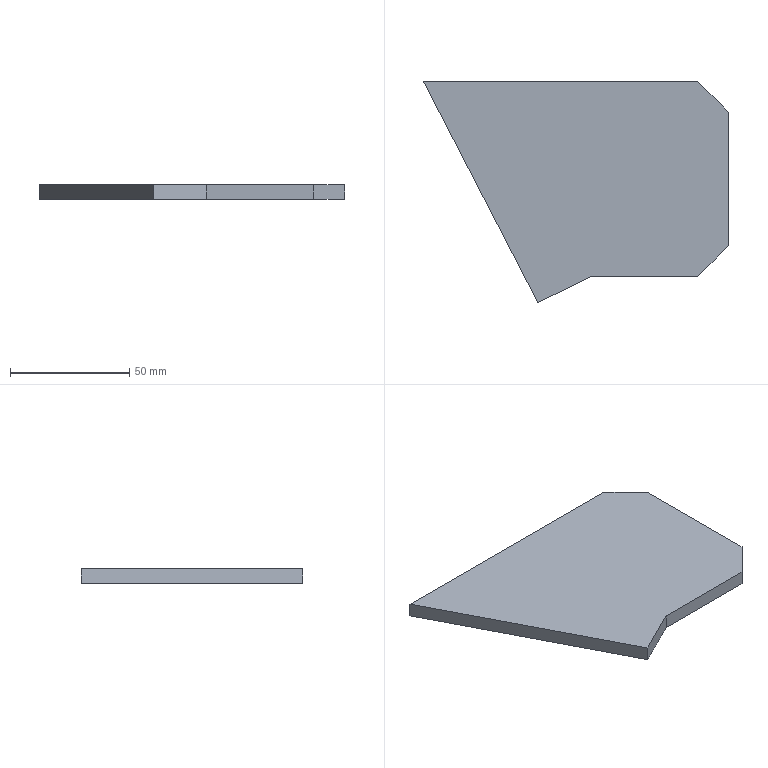Part | SolidWorks | features FlatPattern 1, SMBaseFlange 1, SheetMetal 1 | 1 solid | 9 faces | box 128 x 93 x 6 mm | volume 52464 mm3 | plane 9
STEP:
#1=CARTESIAN_POINT('',(0.,0.,0.));
#2=VERTEX_POINT('',#1);
#3=CARTESIAN_POINT('',(48.,-93.,0.));
#4=VERTEX_POINT('',#3);
#5=CARTESIAN_POINT('',(48.,-93.,0.));
#6=DIRECTION('',(0.4586,-0.8886,0.));
#7=VECTOR('',#6,1000.);
#8=LINE('',#5,#7);
#9=EDGE_CURVE('',#2,#4,#8,.T.);
#10=ORIENTED_EDGE('',*,*,#9,.T.);
#11=CARTESIAN_POINT('',(48.,-93.,6.));
#12=VERTEX_POINT('',#11);
#13=CARTESIAN_POINT('',(48.,-93.,6.));
#14=DIRECTION('',(0.,0.,-1.));
#15=VECTOR('',#14,1000.);
#16=LINE('',#13,#15);
#17=EDGE_CURVE('',#12,#4,#16,.T.);
#18=ORIENTED_EDGE('',*,*,#17,.F.);
#19=CARTESIAN_POINT('',(0.,0.,6.));
#20=VERTEX_POINT('',#19);
#21=CARTESIAN_POINT('',(48.,-93.,6.));
#22=DIRECTION('',(0.4586,-0.8886,0.));
#23=VECTOR('',#22,1000.);
#24=LINE('',#21,#23);
#25=EDGE_CURVE('',#20,#12,#24,.T.);
#26=ORIENTED_EDGE('',*,*,#25,.F.);
#27=CARTESIAN_POINT('',(0.,0.,6.));
#28=DIRECTION('',(0.,0.,-1.));
#29=VECTOR('',#28,1000.);
#30=LINE('',#27,#29);
#31=EDGE_CURVE('',#20,#2,#30,.T.);
#32=ORIENTED_EDGE('',*,*,#31,.T.);
#33=EDGE_LOOP('',(#10,#18,#26,#32));
#34=FACE_OUTER_BOUND('',#33,.T.);
#35=CARTESIAN_POINT('',(48.,-93.,6.));
#36=DIRECTION('',(0.8886,0.4586,0.));
#37=DIRECTION('',(-0.4586,0.8886,0.));
#38=AXIS2_PLACEMENT_3D('',#35,#36,#37);
#39=PLANE('',#38);
#40=ADVANCED_FACE('',(#34),#39,.F.);
#41=CARTESIAN_POINT('',(70.,-82.,0.));
#42=VERTEX_POINT('',#41);
#43=CARTESIAN_POINT('',(70.,-82.,0.));
#44=DIRECTION('',(0.8944,0.4472,0.));
#45=VECTOR('',#44,1000.);
#46=LINE('',#43,#45);
#47=EDGE_CURVE('',#4,#42,#46,.T.);
#48=ORIENTED_EDGE('',*,*,#47,.T.);
#49=CARTESIAN_POINT('',(70.,-82.,6.));
#50=VERTEX_POINT('',#49);
#51=CARTESIAN_POINT('',(70.,-82.,6.));
#52=DIRECTION('',(0.,0.,-1.));
#53=VECTOR('',#52,1000.);
#54=LINE('',#51,#53);
#55=EDGE_CURVE('',#50,#42,#54,.T.);
#56=ORIENTED_EDGE('',*,*,#55,.F.);
#57=CARTESIAN_POINT('',(70.,-82.,6.));
#58=DIRECTION('',(0.8944,0.4472,0.));
#59=VECTOR('',#58,1000.);
#60=LINE('',#57,#59);
#61=EDGE_CURVE('',#12,#50,#60,.T.);
#62=ORIENTED_EDGE('',*,*,#61,.F.);
#63=ORIENTED_EDGE('',*,*,#17,.T.);
#64=EDGE_LOOP('',(#48,#56,#62,#63));
#65=FACE_OUTER_BOUND('',#64,.T.);
#66=CARTESIAN_POINT('',(70.,-82.,6.));
#67=DIRECTION('',(-0.4472,0.8944,0.));
#68=DIRECTION('',(-0.8944,-0.4472,0.));
#69=AXIS2_PLACEMENT_3D('',#66,#67,#68);
#70=PLANE('',#69);
#71=ADVANCED_FACE('',(#65),#70,.F.);
#72=CARTESIAN_POINT('',(115.,-82.,0.));
#73=VERTEX_POINT('',#72);
#74=CARTESIAN_POINT('',(115.,-82.,0.));
#75=DIRECTION('',(1.,0.,0.));
#76=VECTOR('',#75,1000.);
#77=LINE('',#74,#76);
#78=EDGE_CURVE('',#42,#73,#77,.T.);
#79=ORIENTED_EDGE('',*,*,#78,.T.);
#80=CARTESIAN_POINT('',(115.,-82.,6.));
#81=VERTEX_POINT('',#80);
#82=CARTESIAN_POINT('',(115.,-82.,6.));
#83=DIRECTION('',(0.,0.,-1.));
#84=VECTOR('',#83,1000.);
#85=LINE('',#82,#84);
#86=EDGE_CURVE('',#81,#73,#85,.T.);
#87=ORIENTED_EDGE('',*,*,#86,.F.);
#88=CARTESIAN_POINT('',(115.,-82.,6.));
#89=DIRECTION('',(1.,0.,0.));
#90=VECTOR('',#89,1000.);
#91=LINE('',#88,#90);
#92=EDGE_CURVE('',#50,#81,#91,.T.);
#93=ORIENTED_EDGE('',*,*,#92,.F.);
#94=ORIENTED_EDGE('',*,*,#55,.T.);
#95=EDGE_LOOP('',(#79,#87,#93,#94));
#96=FACE_OUTER_BOUND('',#95,.T.);
#97=CARTESIAN_POINT('',(115.,-82.,6.));
#98=DIRECTION('',(0.,1.,0.));
#99=DIRECTION('',(0.,0.,1.));
#100=AXIS2_PLACEMENT_3D('',#97,#98,#99);
#101=PLANE('',#100);
#102=ADVANCED_FACE('',(#96),#101,.F.);
#103=CARTESIAN_POINT('',(128.,-69.,0.));
#104=VERTEX_POINT('',#103);
#105=CARTESIAN_POINT('',(128.,-69.,0.));
#106=DIRECTION('',(0.7071,0.7071,0.));
#107=VECTOR('',#106,1000.);
#108=LINE('',#105,#107);
#109=EDGE_CURVE('',#73,#104,#108,.T.);
#110=ORIENTED_EDGE('',*,*,#109,.T.);
#111=CARTESIAN_POINT('',(128.,-69.,6.));
#112=VERTEX_POINT('',#111);
#113=CARTESIAN_POINT('',(128.,-69.,6.));
#114=DIRECTION('',(0.,0.,-1.));
#115=VECTOR('',#114,1000.);
#116=LINE('',#113,#115);
#117=EDGE_CURVE('',#112,#104,#116,.T.);
#118=ORIENTED_EDGE('',*,*,#117,.F.);
#119=CARTESIAN_POINT('',(128.,-69.,6.));
#120=DIRECTION('',(0.7071,0.7071,0.));
#121=VECTOR('',#120,1000.);
#122=LINE('',#119,#121);
#123=EDGE_CURVE('',#81,#112,#122,.T.);
#124=ORIENTED_EDGE('',*,*,#123,.F.);
#125=ORIENTED_EDGE('',*,*,#86,.T.);
#126=EDGE_LOOP('',(#110,#118,#124,#125));
#127=FACE_OUTER_BOUND('',#126,.T.);
#128=CARTESIAN_POINT('',(128.,-69.,6.));
#129=DIRECTION('',(-0.7071,0.7071,0.));
#130=DIRECTION('',(-0.7071,-0.7071,0.));
#131=AXIS2_PLACEMENT_3D('',#128,#129,#130);
#132=PLANE('',#131);
#133=ADVANCED_FACE('',(#127),#132,.F.);
#134=CARTESIAN_POINT('',(128.,-13.,0.));
#135=VERTEX_POINT('',#134);
#136=CARTESIAN_POINT('',(128.,-13.,0.));
#137=DIRECTION('',(0.,1.,0.));
#138=VECTOR('',#137,1000.);
#139=LINE('',#136,#138);
#140=EDGE_CURVE('',#104,#135,#139,.T.);
#141=ORIENTED_EDGE('',*,*,#140,.T.);
#142=CARTESIAN_POINT('',(128.,-13.,6.));
#143=VERTEX_POINT('',#142);
#144=CARTESIAN_POINT('',(128.,-13.,6.));
#145=DIRECTION('',(0.,0.,-1.));
#146=VECTOR('',#145,1000.);
#147=LINE('',#144,#146);
#148=EDGE_CURVE('',#143,#135,#147,.T.);
#149=ORIENTED_EDGE('',*,*,#148,.F.);
#150=CARTESIAN_POINT('',(128.,-13.,6.));
#151=DIRECTION('',(0.,1.,0.));
#152=VECTOR('',#151,1000.);
#153=LINE('',#150,#152);
#154=EDGE_CURVE('',#112,#143,#153,.T.);
#155=ORIENTED_EDGE('',*,*,#154,.F.);
#156=ORIENTED_EDGE('',*,*,#117,.T.);
#157=EDGE_LOOP('',(#141,#149,#155,#156));
#158=FACE_OUTER_BOUND('',#157,.T.);
#159=CARTESIAN_POINT('',(128.,-13.,6.));
#160=DIRECTION('',(-1.,0.,0.));
#161=DIRECTION('',(0.,0.,1.));
#162=AXIS2_PLACEMENT_3D('',#159,#160,#161);
#163=PLANE('',#162);
#164=ADVANCED_FACE('',(#158),#163,.F.);
#165=CARTESIAN_POINT('',(115.,0.,0.));
#166=VERTEX_POINT('',#165);
#167=CARTESIAN_POINT('',(115.,0.,0.));
#168=DIRECTION('',(-0.7071,0.7071,0.));
#169=VECTOR('',#168,1000.);
#170=LINE('',#167,#169);
#171=EDGE_CURVE('',#135,#166,#170,.T.);
#172=ORIENTED_EDGE('',*,*,#171,.T.);
#173=CARTESIAN_POINT('',(115.,0.,6.));
#174=VERTEX_POINT('',#173);
#175=CARTESIAN_POINT('',(115.,0.,6.));
#176=DIRECTION('',(0.,0.,-1.));
#177=VECTOR('',#176,1000.);
#178=LINE('',#175,#177);
#179=EDGE_CURVE('',#174,#166,#178,.T.);
#180=ORIENTED_EDGE('',*,*,#179,.F.);
#181=CARTESIAN_POINT('',(115.,0.,6.));
#182=DIRECTION('',(-0.7071,0.7071,0.));
#183=VECTOR('',#182,1000.);
#184=LINE('',#181,#183);
#185=EDGE_CURVE('',#143,#174,#184,.T.);
#186=ORIENTED_EDGE('',*,*,#185,.F.);
#187=ORIENTED_EDGE('',*,*,#148,.T.);
#188=EDGE_LOOP('',(#172,#180,#186,#187));
#189=FACE_OUTER_BOUND('',#188,.T.);
#190=CARTESIAN_POINT('',(115.,0.,6.));
#191=DIRECTION('',(-0.7071,-0.7071,0.));
#192=DIRECTION('',(0.7071,-0.7071,0.));
#193=AXIS2_PLACEMENT_3D('',#190,#191,#192);
#194=PLANE('',#193);
#195=ADVANCED_FACE('',(#189),#194,.F.);
#196=CARTESIAN_POINT('',(0.,0.,0.));
#197=DIRECTION('',(-1.,0.,0.));
#198=VECTOR('',#197,1000.);
#199=LINE('',#196,#198);
#200=EDGE_CURVE('',#166,#2,#199,.T.);
#201=ORIENTED_EDGE('',*,*,#200,.T.);
#202=ORIENTED_EDGE('',*,*,#31,.F.);
#203=CARTESIAN_POINT('',(0.,0.,6.));
#204=DIRECTION('',(-1.,0.,0.));
#205=VECTOR('',#204,1000.);
#206=LINE('',#203,#205);
#207=EDGE_CURVE('',#174,#20,#206,.T.);
#208=ORIENTED_EDGE('',*,*,#207,.F.);
#209=ORIENTED_EDGE('',*,*,#179,.T.);
#210=EDGE_LOOP('',(#201,#202,#208,#209));
#211=FACE_OUTER_BOUND('',#210,.T.);
#212=CARTESIAN_POINT('',(0.,0.,6.));
#213=DIRECTION('',(0.,-1.,0.));
#214=DIRECTION('',(0.,0.,-1.));
#215=AXIS2_PLACEMENT_3D('',#212,#213,#214);
#216=PLANE('',#215);
#217=ADVANCED_FACE('',(#211),#216,.F.);
#218=ORIENTED_EDGE('',*,*,#25,.T.);
#219=ORIENTED_EDGE('',*,*,#61,.T.);
#220=ORIENTED_EDGE('',*,*,#92,.T.);
#221=ORIENTED_EDGE('',*,*,#123,.T.);
#222=ORIENTED_EDGE('',*,*,#154,.T.);
#223=ORIENTED_EDGE('',*,*,#185,.T.);
#224=ORIENTED_EDGE('',*,*,#207,.T.);
#225=EDGE_LOOP('',(#218,#219,#220,#221,#222,#223,#224));
#226=FACE_OUTER_BOUND('',#225,.T.);
#227=CARTESIAN_POINT('',(0.,0.,6.));
#228=DIRECTION('',(0.,0.,1.));
#229=DIRECTION('',(1.,0.,0.));
#230=AXIS2_PLACEMENT_3D('',#227,#228,#229);
#231=PLANE('',#230);
#232=ADVANCED_FACE('',(#226),#231,.T.);
#233=ORIENTED_EDGE('',*,*,#9,.F.);
#234=ORIENTED_EDGE('',*,*,#200,.F.);
#235=ORIENTED_EDGE('',*,*,#171,.F.);
#236=ORIENTED_EDGE('',*,*,#140,.F.);
#237=ORIENTED_EDGE('',*,*,#109,.F.);
#238=ORIENTED_EDGE('',*,*,#78,.F.);
#239=ORIENTED_EDGE('',*,*,#47,.F.);
#240=EDGE_LOOP('',(#233,#234,#235,#236,#237,#238,#239));
#241=FACE_OUTER_BOUND('',#240,.T.);
#242=CARTESIAN_POINT('',(0.,0.,0.));
#243=DIRECTION('',(0.,0.,1.));
#244=DIRECTION('',(1.,0.,0.));
#245=AXIS2_PLACEMENT_3D('',#242,#243,#244);
#246=PLANE('',#245);
#247=ADVANCED_FACE('',(#241),#246,.F.);
#248=CLOSED_SHELL('',(#40,#71,#102,#133,#164,#195,#217,#232,#247));
#249=MANIFOLD_SOLID_BREP('',#248);
#250=CARTESIAN_POINT('',(0.,0.,0.));
#251=DIRECTION('',(0.,0.,1.));
#252=DIRECTION('',(1.,0.,0.));
#253=AXIS2_PLACEMENT_3D('',#250,#251,#252);
#254=(LENGTH_UNIT()NAMED_UNIT(*)SI_UNIT(.MILLI.,.METRE.));
#255=UNCERTAINTY_MEASURE_WITH_UNIT(LENGTH_MEASURE(0.00001),#254,'','');
#256=(NAMED_UNIT(*)PLANE_ANGLE_UNIT()SI_UNIT($,.RADIAN.));
#257=(NAMED_UNIT(*)SI_UNIT($,.STERADIAN.)SOLID_ANGLE_UNIT());
#258=(GEOMETRIC_REPRESENTATION_CONTEXT(3)GLOBAL_UNCERTAINTY_ASSIGNED_CONTEXT((#255))GLOBAL_UNIT_ASSIGNED_CONTEXT((#254,#256,#257))REPRESENTATION_CONTEXT('',''));
#259=ADVANCED_BREP_SHAPE_REPRESENTATION('',(#249,#253),#258);